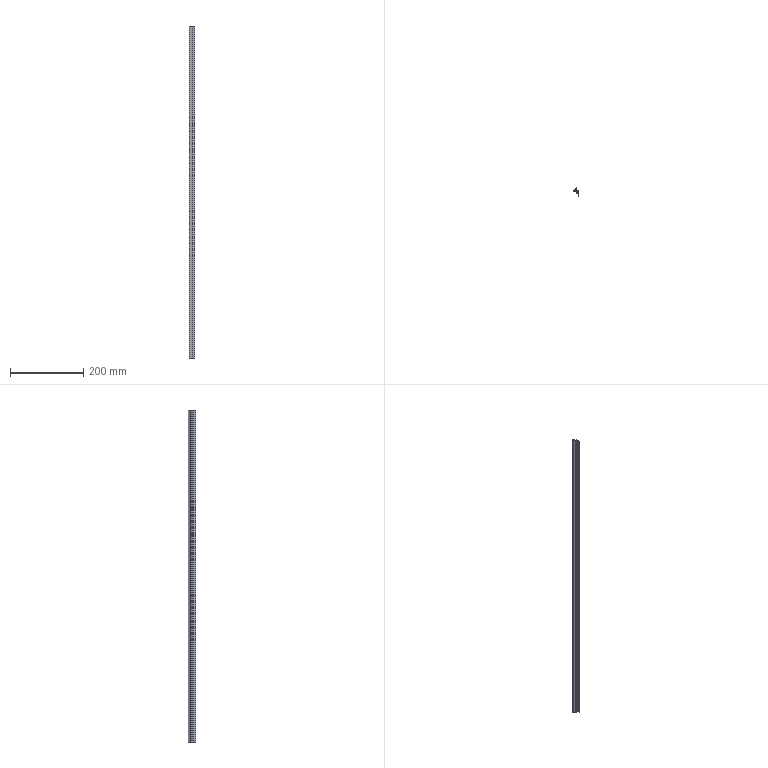Part | SolidWorks | features BaseBody 1, ICE 1, MoveFace 1 | 1 solid | 27 faces | box 14 x 20.3 x 906 mm | volume 46130 mm3 | plane 20 | cylinder 7 | commonest cylinder face diameters 0.387 x2 0.8 x2 0.4 x1 20 x1 22 x1
STEP:
#1=CARTESIAN_POINT('',(-5.304,-0.625,200.));
#2=VERTEX_POINT('',#1);
#3=CARTESIAN_POINT('',(-5.449,-0.8125,200.));
#4=VERTEX_POINT('',#3);
#5=CARTESIAN_POINT('',(-5.255,-0.8125,200.));
#6=DIRECTION('',(0.,0.,1.));
#7=DIRECTION('',(-1.,0.,0.));
#8=AXIS2_PLACEMENT_3D('',#5,#6,#7);
#9=CIRCLE('',#8,0.1937);
#10=EDGE_CURVE('',#2,#4,#9,.T.);
#11=ORIENTED_EDGE('',*,*,#10,.T.);
#12=CARTESIAN_POINT('',(-5.449,-0.8125,-706.));
#13=VERTEX_POINT('',#12);
#14=CARTESIAN_POINT('',(-5.449,-0.8125,230.));
#15=DIRECTION('',(0.,0.,-1.));
#16=VECTOR('',#15,1000.);
#17=LINE('',#14,#16);
#18=EDGE_CURVE('',#4,#13,#17,.T.);
#19=ORIENTED_EDGE('',*,*,#18,.T.);
#20=CARTESIAN_POINT('',(-5.304,-0.625,-706.));
#21=VERTEX_POINT('',#20);
#22=CARTESIAN_POINT('',(-5.255,-0.8125,-706.));
#23=DIRECTION('',(0.,0.,-1.));
#24=DIRECTION('',(1.,0.,0.));
#25=AXIS2_PLACEMENT_3D('',#22,#23,#24);
#26=CIRCLE('',#25,0.1937);
#27=EDGE_CURVE('',#13,#21,#26,.T.);
#28=ORIENTED_EDGE('',*,*,#27,.T.);
#29=CARTESIAN_POINT('',(-5.304,-0.625,230.));
#30=DIRECTION('',(0.,0.,-1.));
#31=VECTOR('',#30,1000.);
#32=LINE('',#29,#31);
#33=EDGE_CURVE('',#2,#21,#32,.T.);
#34=ORIENTED_EDGE('',*,*,#33,.F.);
#35=EDGE_LOOP('',(#11,#19,#28,#34));
#36=FACE_OUTER_BOUND('',#35,.T.);
#37=CARTESIAN_POINT('',(-5.255,-0.8125,230.));
#38=DIRECTION('',(0.,0.,-1.));
#39=DIRECTION('',(-1.,0.,0.));
#40=AXIS2_PLACEMENT_3D('',#37,#38,#39);
#41=CYLINDRICAL_SURFACE('',#40,0.1937);
#42=ADVANCED_FACE('',(#36),#41,.F.);
#43=CARTESIAN_POINT('',(5.,-1.,-706.));
#44=VERTEX_POINT('',#43);
#45=CARTESIAN_POINT('',(5.,-14.3,-706.));
#46=VERTEX_POINT('',#45);
#47=CARTESIAN_POINT('',(5.,29.623,-706.));
#48=DIRECTION('',(0.,-1.,0.));
#49=VECTOR('',#48,1000.);
#50=LINE('',#47,#49);
#51=EDGE_CURVE('',#44,#46,#50,.T.);
#52=ORIENTED_EDGE('',*,*,#51,.F.);
#53=CARTESIAN_POINT('',(5.,-1.,200.));
#54=VERTEX_POINT('',#53);
#55=CARTESIAN_POINT('',(5.,-1.,230.));
#56=DIRECTION('',(0.,0.,-1.));
#57=VECTOR('',#56,1000.);
#58=LINE('',#55,#57);
#59=EDGE_CURVE('',#54,#44,#58,.T.);
#60=ORIENTED_EDGE('',*,*,#59,.F.);
#61=CARTESIAN_POINT('',(5.,-14.3,200.));
#62=VERTEX_POINT('',#61);
#63=CARTESIAN_POINT('',(5.,-14.3,200.));
#64=DIRECTION('',(0.,1.,0.));
#65=VECTOR('',#64,1000.);
#66=LINE('',#63,#65);
#67=EDGE_CURVE('',#62,#54,#66,.T.);
#68=ORIENTED_EDGE('',*,*,#67,.F.);
#69=CARTESIAN_POINT('',(5.,-14.3,230.));
#70=DIRECTION('',(0.,0.,1.));
#71=VECTOR('',#70,1000.);
#72=LINE('',#69,#71);
#73=EDGE_CURVE('',#46,#62,#72,.T.);
#74=ORIENTED_EDGE('',*,*,#73,.F.);
#75=EDGE_LOOP('',(#52,#60,#68,#74));
#76=FACE_OUTER_BOUND('',#75,.T.);
#77=CARTESIAN_POINT('',(5.,-14.3,230.));
#78=DIRECTION('',(-1.,0.,0.));
#79=DIRECTION('',(0.,0.,1.));
#80=AXIS2_PLACEMENT_3D('',#77,#78,#79);
#81=PLANE('',#80);
#82=ADVANCED_FACE('',(#76),#81,.F.);
#83=CARTESIAN_POINT('',(-9.,-2.,-706.));
#84=VERTEX_POINT('',#83);
#85=CARTESIAN_POINT('',(-9.,-2.,200.));
#86=VERTEX_POINT('',#85);
#87=CARTESIAN_POINT('',(-9.,-2.,230.));
#88=DIRECTION('',(0.,0.,1.));
#89=VECTOR('',#88,1000.);
#90=LINE('',#87,#89);
#91=EDGE_CURVE('',#84,#86,#90,.T.);
#92=ORIENTED_EDGE('',*,*,#91,.F.);
#93=CARTESIAN_POINT('',(0.9,-2.,-706.));
#94=VERTEX_POINT('',#93);
#95=CARTESIAN_POINT('',(5.,-2.,-706.));
#96=DIRECTION('',(-1.,0.,0.));
#97=VECTOR('',#96,1000.);
#98=LINE('',#95,#97);
#99=EDGE_CURVE('',#94,#84,#98,.T.);
#100=ORIENTED_EDGE('',*,*,#99,.F.);
#101=CARTESIAN_POINT('',(0.9,-2.,200.));
#102=VERTEX_POINT('',#101);
#103=CARTESIAN_POINT('',(0.9,-2.,230.));
#104=DIRECTION('',(0.,0.,-1.));
#105=VECTOR('',#104,1000.);
#106=LINE('',#103,#105);
#107=EDGE_CURVE('',#102,#94,#106,.T.);
#108=ORIENTED_EDGE('',*,*,#107,.F.);
#109=CARTESIAN_POINT('',(5.,-2.,200.));
#110=DIRECTION('',(1.,0.,0.));
#111=VECTOR('',#110,1000.);
#112=LINE('',#109,#111);
#113=EDGE_CURVE('',#86,#102,#112,.T.);
#114=ORIENTED_EDGE('',*,*,#113,.F.);
#115=EDGE_LOOP('',(#92,#100,#108,#114));
#116=FACE_OUTER_BOUND('',#115,.T.);
#117=CARTESIAN_POINT('',(-9.,-2.,230.));
#118=DIRECTION('',(0.,1.,0.));
#119=DIRECTION('',(0.,0.,1.));
#120=AXIS2_PLACEMENT_3D('',#117,#118,#119);
#121=PLANE('',#120);
#122=ADVANCED_FACE('',(#116),#121,.F.);
#123=CARTESIAN_POINT('',(4.,-6.,200.));
#124=VERTEX_POINT('',#123);
#125=CARTESIAN_POINT('',(4.,-3.,200.));
#126=VERTEX_POINT('',#125);
#127=CARTESIAN_POINT('',(4.,29.623,200.));
#128=DIRECTION('',(0.,1.,0.));
#129=VECTOR('',#128,1000.);
#130=LINE('',#127,#129);
#131=EDGE_CURVE('',#124,#126,#130,.T.);
#132=ORIENTED_EDGE('',*,*,#131,.F.);
#133=CARTESIAN_POINT('',(1.,-6.,200.));
#134=VERTEX_POINT('',#133);
#135=CARTESIAN_POINT('',(5.,-6.,200.));
#136=DIRECTION('',(1.,0.,0.));
#137=VECTOR('',#136,1000.);
#138=LINE('',#135,#137);
#139=EDGE_CURVE('',#134,#124,#138,.T.);
#140=ORIENTED_EDGE('',*,*,#139,.F.);
#141=CARTESIAN_POINT('',(1.,-6.7,200.));
#142=VERTEX_POINT('',#141);
#143=CARTESIAN_POINT('',(1.,-6.,200.));
#144=DIRECTION('',(0.,-1.,0.));
#145=VECTOR('',#144,1000.);
#146=LINE('',#143,#145);
#147=EDGE_CURVE('',#134,#142,#146,.T.);
#148=ORIENTED_EDGE('',*,*,#147,.T.);
#149=CARTESIAN_POINT('',(-1.7,-6.7,200.));
#150=VERTEX_POINT('',#149);
#151=CARTESIAN_POINT('',(5.,-6.7,200.));
#152=DIRECTION('',(1.,0.,0.));
#153=VECTOR('',#152,1000.);
#154=LINE('',#151,#153);
#155=EDGE_CURVE('',#150,#142,#154,.T.);
#156=ORIENTED_EDGE('',*,*,#155,.F.);
#157=CARTESIAN_POINT('',(-1.7,-7.7,200.));
#158=VERTEX_POINT('',#157);
#159=CARTESIAN_POINT('',(-1.7,-6.7,200.));
#160=DIRECTION('',(0.,-1.,0.));
#161=VECTOR('',#160,1000.);
#162=LINE('',#159,#161);
#163=EDGE_CURVE('',#150,#158,#162,.T.);
#164=ORIENTED_EDGE('',*,*,#163,.T.);
#165=CARTESIAN_POINT('',(4.,-7.7,200.));
#166=VERTEX_POINT('',#165);
#167=CARTESIAN_POINT('',(5.,-7.7,200.));
#168=DIRECTION('',(-1.,0.,0.));
#169=VECTOR('',#168,1000.);
#170=LINE('',#167,#169);
#171=EDGE_CURVE('',#166,#158,#170,.T.);
#172=ORIENTED_EDGE('',*,*,#171,.F.);
#173=CARTESIAN_POINT('',(4.,-14.3,200.));
#174=VERTEX_POINT('',#173);
#175=CARTESIAN_POINT('',(4.,29.623,200.));
#176=DIRECTION('',(0.,1.,0.));
#177=VECTOR('',#176,1000.);
#178=LINE('',#175,#177);
#179=EDGE_CURVE('',#174,#166,#178,.T.);
#180=ORIENTED_EDGE('',*,*,#179,.F.);
#181=CARTESIAN_POINT('',(5.,-14.3,200.));
#182=DIRECTION('',(-1.,0.,0.));
#183=VECTOR('',#182,1000.);
#184=LINE('',#181,#183);
#185=EDGE_CURVE('',#62,#174,#184,.T.);
#186=ORIENTED_EDGE('',*,*,#185,.F.);
#187=ORIENTED_EDGE('',*,*,#67,.T.);
#188=CARTESIAN_POINT('',(-5.207,-1.,200.));
#189=VERTEX_POINT('',#188);
#190=CARTESIAN_POINT('',(5.,-1.,200.));
#191=DIRECTION('',(1.,0.,0.));
#192=VECTOR('',#191,1000.);
#193=LINE('',#190,#192);
#194=EDGE_CURVE('',#189,#54,#193,.T.);
#195=ORIENTED_EDGE('',*,*,#194,.F.);
#196=CARTESIAN_POINT('',(-5.255,-0.8125,200.));
#197=DIRECTION('',(0.,0.,1.));
#198=DIRECTION('',(-1.,0.,0.));
#199=AXIS2_PLACEMENT_3D('',#196,#197,#198);
#200=CIRCLE('',#199,0.1937);
#201=EDGE_CURVE('',#4,#189,#200,.T.);
#202=ORIENTED_EDGE('',*,*,#201,.F.);
#203=ORIENTED_EDGE('',*,*,#10,.F.);
#204=CARTESIAN_POINT('',(-1.368,3.063,200.));
#205=VERTEX_POINT('',#204);
#206=CARTESIAN_POINT('',(-10.628,9.,200.));
#207=DIRECTION('',(0.,0.,1.));
#208=DIRECTION('',(-1.,0.,0.));
#209=AXIS2_PLACEMENT_3D('',#206,#207,#208);
#210=CIRCLE('',#209,11.);
#211=EDGE_CURVE('',#2,#205,#210,.T.);
#212=ORIENTED_EDGE('',*,*,#211,.T.);
#213=CARTESIAN_POINT('',(-1.,2.955,200.));
#214=VERTEX_POINT('',#213);
#215=CARTESIAN_POINT('',(-1.2,2.955,200.));
#216=DIRECTION('',(0.,0.,1.));
#217=DIRECTION('',(-1.,0.,0.));
#218=AXIS2_PLACEMENT_3D('',#215,#216,#217);
#219=CIRCLE('',#218,0.2);
#220=EDGE_CURVE('',#214,#205,#219,.T.);
#221=ORIENTED_EDGE('',*,*,#220,.F.);
#222=CARTESIAN_POINT('',(-1.,1.5,200.));
#223=VERTEX_POINT('',#222);
#224=CARTESIAN_POINT('',(-1.,2.955,200.));
#225=DIRECTION('',(0.,1.,0.));
#226=VECTOR('',#225,1000.);
#227=LINE('',#224,#226);
#228=EDGE_CURVE('',#223,#214,#227,.T.);
#229=ORIENTED_EDGE('',*,*,#228,.F.);
#230=CARTESIAN_POINT('',(0.,1.5,200.));
#231=VERTEX_POINT('',#230);
#232=CARTESIAN_POINT('',(-1.,1.5,200.));
#233=DIRECTION('',(-1.,0.,0.));
#234=VECTOR('',#233,1000.);
#235=LINE('',#232,#234);
#236=EDGE_CURVE('',#231,#223,#235,.T.);
#237=ORIENTED_EDGE('',*,*,#236,.F.);
#238=CARTESIAN_POINT('',(0.,6.,200.));
#239=VERTEX_POINT('',#238);
#240=CARTESIAN_POINT('',(0.,1.5,200.));
#241=DIRECTION('',(0.,-1.,0.));
#242=VECTOR('',#241,1000.);
#243=LINE('',#240,#242);
#244=EDGE_CURVE('',#239,#231,#243,.T.);
#245=ORIENTED_EDGE('',*,*,#244,.F.);
#246=CARTESIAN_POINT('',(-0.8,6.,200.));
#247=VERTEX_POINT('',#246);
#248=CARTESIAN_POINT('',(0.,6.,200.));
#249=DIRECTION('',(1.,0.,0.));
#250=VECTOR('',#249,1000.);
#251=LINE('',#248,#250);
#252=EDGE_CURVE('',#247,#239,#251,.T.);
#253=ORIENTED_EDGE('',*,*,#252,.F.);
#254=CARTESIAN_POINT('',(-1.178,5.731,200.));
#255=VERTEX_POINT('',#254);
#256=CARTESIAN_POINT('',(-0.8,5.6,200.));
#257=DIRECTION('',(0.,0.,1.));
#258=DIRECTION('',(-1.,0.,0.));
#259=AXIS2_PLACEMENT_3D('',#256,#257,#258);
#260=CIRCLE('',#259,0.4);
#261=EDGE_CURVE('',#247,#255,#260,.T.);
#262=ORIENTED_EDGE('',*,*,#261,.T.);
#263=CARTESIAN_POINT('',(-8.678,-0.8077,200.));
#264=VERTEX_POINT('',#263);
#265=CARTESIAN_POINT('',(-10.628,9.,200.));
#266=DIRECTION('',(0.,0.,1.));
#267=DIRECTION('',(-1.,0.,0.));
#268=AXIS2_PLACEMENT_3D('',#265,#266,#267);
#269=CIRCLE('',#268,10.);
#270=EDGE_CURVE('',#264,#255,#269,.T.);
#271=ORIENTED_EDGE('',*,*,#270,.F.);
#272=CARTESIAN_POINT('',(-9.,-1.2,200.));
#273=VERTEX_POINT('',#272);
#274=CARTESIAN_POINT('',(-8.6,-1.2,200.));
#275=DIRECTION('',(0.,0.,1.));
#276=DIRECTION('',(-1.,0.,0.));
#277=AXIS2_PLACEMENT_3D('',#274,#275,#276);
#278=CIRCLE('',#277,0.4);
#279=EDGE_CURVE('',#264,#273,#278,.T.);
#280=ORIENTED_EDGE('',*,*,#279,.T.);
#281=CARTESIAN_POINT('',(-9.,8.,200.));
#282=DIRECTION('',(0.,-1.,0.));
#283=VECTOR('',#282,1000.);
#284=LINE('',#281,#283);
#285=EDGE_CURVE('',#273,#86,#284,.T.);
#286=ORIENTED_EDGE('',*,*,#285,.T.);
#287=ORIENTED_EDGE('',*,*,#113,.T.);
#288=CARTESIAN_POINT('',(0.9,-3.,200.));
#289=VERTEX_POINT('',#288);
#290=CARTESIAN_POINT('',(0.9,29.623,200.));
#291=DIRECTION('',(0.,1.,0.));
#292=VECTOR('',#291,1000.);
#293=LINE('',#290,#292);
#294=EDGE_CURVE('',#289,#102,#293,.T.);
#295=ORIENTED_EDGE('',*,*,#294,.F.);
#296=CARTESIAN_POINT('',(5.,-3.,200.));
#297=DIRECTION('',(-1.,0.,0.));
#298=VECTOR('',#297,1000.);
#299=LINE('',#296,#298);
#300=EDGE_CURVE('',#126,#289,#299,.T.);
#301=ORIENTED_EDGE('',*,*,#300,.F.);
#302=EDGE_LOOP('',(#132,#140,#148,#156,#164,#172,#180,#186,#187,#195,#202,#203,#212,#221,#229,#237,#245,#253,#262,#271,#280,#286,#287,#295,#301));
#303=FACE_OUTER_BOUND('',#302,.T.);
#304=CARTESIAN_POINT('',(5.,29.623,200.));
#305=DIRECTION('',(0.,0.,-1.));
#306=DIRECTION('',(-1.,0.,0.));
#307=AXIS2_PLACEMENT_3D('',#304,#305,#306);
#308=PLANE('',#307);
#309=ADVANCED_FACE('',(#303),#308,.F.);
#310=ORIENTED_EDGE('',*,*,#185,.T.);
#311=CARTESIAN_POINT('',(4.,-14.3,-706.));
#312=VERTEX_POINT('',#311);
#313=CARTESIAN_POINT('',(4.,-14.3,230.));
#314=DIRECTION('',(0.,0.,1.));
#315=VECTOR('',#314,1000.);
#316=LINE('',#313,#315);
#317=EDGE_CURVE('',#312,#174,#316,.T.);
#318=ORIENTED_EDGE('',*,*,#317,.F.);
#319=CARTESIAN_POINT('',(5.,-14.3,-706.));
#320=DIRECTION('',(-1.,0.,0.));
#321=VECTOR('',#320,1000.);
#322=LINE('',#319,#321);
#323=EDGE_CURVE('',#46,#312,#322,.T.);
#324=ORIENTED_EDGE('',*,*,#323,.F.);
#325=ORIENTED_EDGE('',*,*,#73,.T.);
#326=EDGE_LOOP('',(#310,#318,#324,#325));
#327=FACE_OUTER_BOUND('',#326,.T.);
#328=CARTESIAN_POINT('',(4.,-14.3,230.));
#329=DIRECTION('',(0.,1.,0.));
#330=DIRECTION('',(0.,0.,1.));
#331=AXIS2_PLACEMENT_3D('',#328,#329,#330);
#332=PLANE('',#331);
#333=ADVANCED_FACE('',(#327),#332,.F.);
#334=ORIENTED_EDGE('',*,*,#51,.T.);
#335=ORIENTED_EDGE('',*,*,#323,.T.);
#336=CARTESIAN_POINT('',(4.,-7.7,-706.));
#337=VERTEX_POINT('',#336);
#338=CARTESIAN_POINT('',(4.,-7.7,-706.));
#339=DIRECTION('',(0.,-1.,0.));
#340=VECTOR('',#339,1000.);
#341=LINE('',#338,#340);
#342=EDGE_CURVE('',#337,#312,#341,.T.);
#343=ORIENTED_EDGE('',*,*,#342,.F.);
#344=CARTESIAN_POINT('',(-1.7,-7.7,-706.));
#345=VERTEX_POINT('',#344);
#346=CARTESIAN_POINT('',(-1.7,-7.7,-706.));
#347=DIRECTION('',(1.,0.,0.));
#348=VECTOR('',#347,1000.);
#349=LINE('',#346,#348);
#350=EDGE_CURVE('',#345,#337,#349,.T.);
#351=ORIENTED_EDGE('',*,*,#350,.F.);
#352=CARTESIAN_POINT('',(-1.7,-6.7,-706.));
#353=VERTEX_POINT('',#352);
#354=CARTESIAN_POINT('',(-1.7,29.623,-706.));
#355=DIRECTION('',(0.,1.,0.));
#356=VECTOR('',#355,1000.);
#357=LINE('',#354,#356);
#358=EDGE_CURVE('',#345,#353,#357,.T.);
#359=ORIENTED_EDGE('',*,*,#358,.T.);
#360=CARTESIAN_POINT('',(1.,-6.7,-706.));
#361=VERTEX_POINT('',#360);
#362=CARTESIAN_POINT('',(1.,-6.7,-706.));
#363=DIRECTION('',(-1.,0.,0.));
#364=VECTOR('',#363,1000.);
#365=LINE('',#362,#364);
#366=EDGE_CURVE('',#361,#353,#365,.T.);
#367=ORIENTED_EDGE('',*,*,#366,.F.);
#368=CARTESIAN_POINT('',(1.,-6.,-706.));
#369=VERTEX_POINT('',#368);
#370=CARTESIAN_POINT('',(1.,29.623,-706.));
#371=DIRECTION('',(0.,1.,0.));
#372=VECTOR('',#371,1000.);
#373=LINE('',#370,#372);
#374=EDGE_CURVE('',#361,#369,#373,.T.);
#375=ORIENTED_EDGE('',*,*,#374,.T.);
#376=CARTESIAN_POINT('',(4.,-6.,-706.));
#377=VERTEX_POINT('',#376);
#378=CARTESIAN_POINT('',(4.,-6.,-706.));
#379=DIRECTION('',(-1.,0.,0.));
#380=VECTOR('',#379,1000.);
#381=LINE('',#378,#380);
#382=EDGE_CURVE('',#377,#369,#381,.T.);
#383=ORIENTED_EDGE('',*,*,#382,.F.);
#384=CARTESIAN_POINT('',(4.,-3.,-706.));
#385=VERTEX_POINT('',#384);
#386=CARTESIAN_POINT('',(4.,-3.,-706.));
#387=DIRECTION('',(0.,-1.,0.));
#388=VECTOR('',#387,1000.);
#389=LINE('',#386,#388);
#390=EDGE_CURVE('',#385,#377,#389,.T.);
#391=ORIENTED_EDGE('',*,*,#390,.F.);
#392=CARTESIAN_POINT('',(0.9,-3.,-706.));
#393=VERTEX_POINT('',#392);
#394=CARTESIAN_POINT('',(0.9,-3.,-706.));
#395=DIRECTION('',(1.,0.,0.));
#396=VECTOR('',#395,1000.);
#397=LINE('',#394,#396);
#398=EDGE_CURVE('',#393,#385,#397,.T.);
#399=ORIENTED_EDGE('',*,*,#398,.F.);
#400=CARTESIAN_POINT('',(0.9,-2.,-706.));
#401=DIRECTION('',(0.,-1.,0.));
#402=VECTOR('',#401,1000.);
#403=LINE('',#400,#402);
#404=EDGE_CURVE('',#94,#393,#403,.T.);
#405=ORIENTED_EDGE('',*,*,#404,.F.);
#406=ORIENTED_EDGE('',*,*,#99,.T.);
#407=CARTESIAN_POINT('',(-9.,-1.2,-706.));
#408=VERTEX_POINT('',#407);
#409=CARTESIAN_POINT('',(-9.,-1.2,-706.));
#410=DIRECTION('',(0.,-1.,0.));
#411=VECTOR('',#410,1000.);
#412=LINE('',#409,#411);
#413=EDGE_CURVE('',#408,#84,#412,.T.);
#414=ORIENTED_EDGE('',*,*,#413,.F.);
#415=CARTESIAN_POINT('',(-8.678,-0.8077,-706.));
#416=VERTEX_POINT('',#415);
#417=CARTESIAN_POINT('',(-8.6,-1.2,-706.));
#418=DIRECTION('',(0.,0.,-1.));
#419=DIRECTION('',(1.,0.,0.));
#420=AXIS2_PLACEMENT_3D('',#417,#418,#419);
#421=CIRCLE('',#420,0.4);
#422=EDGE_CURVE('',#408,#416,#421,.T.);
#423=ORIENTED_EDGE('',*,*,#422,.T.);
#424=CARTESIAN_POINT('',(-1.178,5.731,-706.));
#425=VERTEX_POINT('',#424);
#426=CARTESIAN_POINT('',(-10.628,9.,-706.));
#427=DIRECTION('',(0.,0.,-1.));
#428=DIRECTION('',(1.,0.,0.));
#429=AXIS2_PLACEMENT_3D('',#426,#427,#428);
#430=CIRCLE('',#429,10.);
#431=EDGE_CURVE('',#425,#416,#430,.T.);
#432=ORIENTED_EDGE('',*,*,#431,.F.);
#433=CARTESIAN_POINT('',(-0.8,6.,-706.));
#434=VERTEX_POINT('',#433);
#435=CARTESIAN_POINT('',(-0.8,5.6,-706.));
#436=DIRECTION('',(0.,0.,-1.));
#437=DIRECTION('',(1.,0.,0.));
#438=AXIS2_PLACEMENT_3D('',#435,#436,#437);
#439=CIRCLE('',#438,0.4);
#440=EDGE_CURVE('',#425,#434,#439,.T.);
#441=ORIENTED_EDGE('',*,*,#440,.T.);
#442=CARTESIAN_POINT('',(0.,6.,-706.));
#443=VERTEX_POINT('',#442);
#444=CARTESIAN_POINT('',(0.,6.,-706.));
#445=DIRECTION('',(-1.,0.,0.));
#446=VECTOR('',#445,1000.);
#447=LINE('',#444,#446);
#448=EDGE_CURVE('',#443,#434,#447,.T.);
#449=ORIENTED_EDGE('',*,*,#448,.F.);
#450=CARTESIAN_POINT('',(0.,1.5,-706.));
#451=VERTEX_POINT('',#450);
#452=CARTESIAN_POINT('',(0.,1.5,-706.));
#453=DIRECTION('',(0.,1.,0.));
#454=VECTOR('',#453,1000.);
#455=LINE('',#452,#454);
#456=EDGE_CURVE('',#451,#443,#455,.T.);
#457=ORIENTED_EDGE('',*,*,#456,.F.);
#458=CARTESIAN_POINT('',(-1.,1.5,-706.));
#459=VERTEX_POINT('',#458);
#460=CARTESIAN_POINT('',(-1.,1.5,-706.));
#461=DIRECTION('',(1.,0.,0.));
#462=VECTOR('',#461,1000.);
#463=LINE('',#460,#462);
#464=EDGE_CURVE('',#459,#451,#463,.T.);
#465=ORIENTED_EDGE('',*,*,#464,.F.);
#466=CARTESIAN_POINT('',(-1.,2.955,-706.));
#467=VERTEX_POINT('',#466);
#468=CARTESIAN_POINT('',(-1.,2.955,-706.));
#469=DIRECTION('',(0.,-1.,0.));
#470=VECTOR('',#469,1000.);
#471=LINE('',#468,#470);
#472=EDGE_CURVE('',#467,#459,#471,.T.);
#473=ORIENTED_EDGE('',*,*,#472,.F.);
#474=CARTESIAN_POINT('',(-1.368,3.063,-706.));
#475=VERTEX_POINT('',#474);
#476=CARTESIAN_POINT('',(-1.2,2.955,-706.));
#477=DIRECTION('',(0.,0.,-1.));
#478=DIRECTION('',(1.,0.,0.));
#479=AXIS2_PLACEMENT_3D('',#476,#477,#478);
#480=CIRCLE('',#479,0.2);
#481=EDGE_CURVE('',#475,#467,#480,.T.);
#482=ORIENTED_EDGE('',*,*,#481,.F.);
#483=CARTESIAN_POINT('',(-10.628,9.,-706.));
#484=DIRECTION('',(0.,0.,-1.));
#485=DIRECTION('',(1.,0.,0.));
#486=AXIS2_PLACEMENT_3D('',#483,#484,#485);
#487=CIRCLE('',#486,11.);
#488=EDGE_CURVE('',#475,#21,#487,.T.);
#489=ORIENTED_EDGE('',*,*,#488,.T.);
#490=ORIENTED_EDGE('',*,*,#27,.F.);
#491=CARTESIAN_POINT('',(-5.207,-1.,-706.));
#492=VERTEX_POINT('',#491);
#493=CARTESIAN_POINT('',(-5.255,-0.8125,-706.));
#494=DIRECTION('',(0.,0.,-1.));
#495=DIRECTION('',(1.,0.,0.));
#496=AXIS2_PLACEMENT_3D('',#493,#494,#495);
#497=CIRCLE('',#496,0.1937);
#498=EDGE_CURVE('',#492,#13,#497,.T.);
#499=ORIENTED_EDGE('',*,*,#498,.F.);
#500=CARTESIAN_POINT('',(5.,-1.,-706.));
#501=DIRECTION('',(-1.,0.,0.));
#502=VECTOR('',#501,1000.);
#503=LINE('',#500,#502);
#504=EDGE_CURVE('',#44,#492,#503,.T.);
#505=ORIENTED_EDGE('',*,*,#504,.F.);
#506=EDGE_LOOP('',(#334,#335,#343,#351,#359,#367,#375,#383,#391,#399,#405,#406,#414,#423,#432,#441,#449,#457,#465,#473,#482,#489,#490,#499,#505));
#507=FACE_OUTER_BOUND('',#506,.T.);
#508=CARTESIAN_POINT('',(5.,29.623,-706.));
#509=DIRECTION('',(0.,0.,1.));
#510=DIRECTION('',(1.,0.,0.));
#511=AXIS2_PLACEMENT_3D('',#508,#509,#510);
#512=PLANE('',#511);
#513=ADVANCED_FACE('',(#507),#512,.F.);
#514=ORIENTED_EDGE('',*,*,#59,.T.);
#515=ORIENTED_EDGE('',*,*,#504,.T.);
#516=CARTESIAN_POINT('',(-5.207,-1.,230.));
#517=DIRECTION('',(0.,0.,-1.));
#518=VECTOR('',#517,1000.);
#519=LINE('',#516,#518);
#520=EDGE_CURVE('',#189,#492,#519,.T.);
#521=ORIENTED_EDGE('',*,*,#520,.F.);
#522=ORIENTED_EDGE('',*,*,#194,.T.);
#523=EDGE_LOOP('',(#514,#515,#521,#522));
#524=FACE_OUTER_BOUND('',#523,.T.);
#525=CARTESIAN_POINT('',(5.,-1.,230.));
#526=DIRECTION('',(0.,-1.,0.));
#527=DIRECTION('',(0.,0.,-1.));
#528=AXIS2_PLACEMENT_3D('',#525,#526,#527);
#529=PLANE('',#528);
#530=ADVANCED_FACE('',(#524),#529,.F.);
#531=CARTESIAN_POINT('',(-9.,-1.2,230.));
#532=DIRECTION('',(0.,0.,1.));
#533=VECTOR('',#532,1000.);
#534=LINE('',#531,#533);
#535=EDGE_CURVE('',#408,#273,#534,.T.);
#536=ORIENTED_EDGE('',*,*,#535,.F.);
#537=ORIENTED_EDGE('',*,*,#413,.T.);
#538=ORIENTED_EDGE('',*,*,#91,.T.);
#539=ORIENTED_EDGE('',*,*,#285,.F.);
#540=EDGE_LOOP('',(#536,#537,#538,#539));
#541=FACE_OUTER_BOUND('',#540,.T.);
#542=CARTESIAN_POINT('',(-9.,-1.2,230.));
#543=DIRECTION('',(1.,0.,0.));
#544=DIRECTION('',(0.,0.,-1.));
#545=AXIS2_PLACEMENT_3D('',#542,#543,#544);
#546=PLANE('',#545);
#547=ADVANCED_FACE('',(#541),#546,.F.);
#548=ORIENTED_EDGE('',*,*,#294,.T.);
#549=ORIENTED_EDGE('',*,*,#107,.T.);
#550=ORIENTED_EDGE('',*,*,#404,.T.);
#551=CARTESIAN_POINT('',(0.9,-3.,230.));
#552=DIRECTION('',(0.,0.,-1.));
#553=VECTOR('',#552,1000.);
#554=LINE('',#551,#553);
#555=EDGE_CURVE('',#289,#393,#554,.T.);
#556=ORIENTED_EDGE('',*,*,#555,.F.);
#557=EDGE_LOOP('',(#548,#549,#550,#556));
#558=FACE_OUTER_BOUND('',#557,.T.);
#559=CARTESIAN_POINT('',(0.9,-2.,230.));
#560=DIRECTION('',(1.,0.,0.));
#561=DIRECTION('',(0.,0.,-1.));
#562=AXIS2_PLACEMENT_3D('',#559,#560,#561);
#563=PLANE('',#562);
#564=ADVANCED_FACE('',(#558),#563,.F.);
#565=ORIENTED_EDGE('',*,*,#300,.T.);
#566=ORIENTED_EDGE('',*,*,#555,.T.);
#567=ORIENTED_EDGE('',*,*,#398,.T.);
#568=CARTESIAN_POINT('',(4.,-3.,230.));
#569=DIRECTION('',(0.,0.,-1.));
#570=VECTOR('',#569,1000.);
#571=LINE('',#568,#570);
#572=EDGE_CURVE('',#126,#385,#571,.T.);
#573=ORIENTED_EDGE('',*,*,#572,.F.);
#574=EDGE_LOOP('',(#565,#566,#567,#573));
#575=FACE_OUTER_BOUND('',#574,.T.);
#576=CARTESIAN_POINT('',(0.9,-3.,230.));
#577=DIRECTION('',(0.,1.,0.));
#578=DIRECTION('',(0.,0.,1.));
#579=AXIS2_PLACEMENT_3D('',#576,#577,#578);
#580=PLANE('',#579);
#581=ADVANCED_FACE('',(#575),#580,.F.);
#582=ORIENTED_EDGE('',*,*,#131,.T.);
#583=ORIENTED_EDGE('',*,*,#572,.T.);
#584=ORIENTED_EDGE('',*,*,#390,.T.);
#585=CARTESIAN_POINT('',(4.,-6.,230.));
#586=DIRECTION('',(0.,0.,-1.));
#587=VECTOR('',#586,1000.);
#588=LINE('',#585,#587);
#589=EDGE_CURVE('',#124,#377,#588,.T.);
#590=ORIENTED_EDGE('',*,*,#589,.F.);
#591=EDGE_LOOP('',(#582,#583,#584,#590));
#592=FACE_OUTER_BOUND('',#591,.T.);
#593=CARTESIAN_POINT('',(4.,-3.,230.));
#594=DIRECTION('',(1.,0.,0.));
#595=DIRECTION('',(0.,0.,-1.));
#596=AXIS2_PLACEMENT_3D('',#593,#594,#595);
#597=PLANE('',#596);
#598=ADVANCED_FACE('',(#592),#597,.F.);
#599=ORIENTED_EDGE('',*,*,#139,.T.);
#600=ORIENTED_EDGE('',*,*,#589,.T.);
#601=ORIENTED_EDGE('',*,*,#382,.T.);
#602=CARTESIAN_POINT('',(1.,-6.,230.));
#603=DIRECTION('',(0.,0.,-1.));
#604=VECTOR('',#603,1000.);
#605=LINE('',#602,#604);
#606=EDGE_CURVE('',#134,#369,#605,.T.);
#607=ORIENTED_EDGE('',*,*,#606,.F.);
#608=EDGE_LOOP('',(#599,#600,#601,#607));
#609=FACE_OUTER_BOUND('',#608,.T.);
#610=CARTESIAN_POINT('',(4.,-6.,230.));
#611=DIRECTION('',(0.,-1.,0.));
#612=DIRECTION('',(0.,0.,-1.));
#613=AXIS2_PLACEMENT_3D('',#610,#611,#612);
#614=PLANE('',#613);
#615=ADVANCED_FACE('',(#609),#614,.F.);
#616=ORIENTED_EDGE('',*,*,#155,.T.);
#617=CARTESIAN_POINT('',(1.,-6.7,230.));
#618=DIRECTION('',(0.,0.,1.));
#619=VECTOR('',#618,1000.);
#620=LINE('',#617,#619);
#621=EDGE_CURVE('',#361,#142,#620,.T.);
#622=ORIENTED_EDGE('',*,*,#621,.F.);
#623=ORIENTED_EDGE('',*,*,#366,.T.);
#624=CARTESIAN_POINT('',(-1.7,-6.7,230.));
#625=DIRECTION('',(0.,0.,-1.));
#626=VECTOR('',#625,1000.);
#627=LINE('',#624,#626);
#628=EDGE_CURVE('',#150,#353,#627,.T.);
#629=ORIENTED_EDGE('',*,*,#628,.F.);
#630=EDGE_LOOP('',(#616,#622,#623,#629));
#631=FACE_OUTER_BOUND('',#630,.T.);
#632=CARTESIAN_POINT('',(1.,-6.7,230.));
#633=DIRECTION('',(0.,-1.,0.));
#634=DIRECTION('',(0.,0.,-1.));
#635=AXIS2_PLACEMENT_3D('',#632,#633,#634);
#636=PLANE('',#635);
#637=ADVANCED_FACE('',(#631),#636,.F.);
#638=ORIENTED_EDGE('',*,*,#171,.T.);
#639=CARTESIAN_POINT('',(-1.7,-7.7,230.));
#640=DIRECTION('',(0.,0.,1.));
#641=VECTOR('',#640,1000.);
#642=LINE('',#639,#641);
#643=EDGE_CURVE('',#345,#158,#642,.T.);
#644=ORIENTED_EDGE('',*,*,#643,.F.);
#645=ORIENTED_EDGE('',*,*,#350,.T.);
#646=CARTESIAN_POINT('',(4.,-7.7,230.));
#647=DIRECTION('',(0.,0.,-1.));
#648=VECTOR('',#647,1000.);
#649=LINE('',#646,#648);
#650=EDGE_CURVE('',#166,#337,#649,.T.);
#651=ORIENTED_EDGE('',*,*,#650,.F.);
#652=EDGE_LOOP('',(#638,#644,#645,#651));
#653=FACE_OUTER_BOUND('',#652,.T.);
#654=CARTESIAN_POINT('',(-1.7,-7.7,230.));
#655=DIRECTION('',(0.,1.,0.));
#656=DIRECTION('',(0.,0.,1.));
#657=AXIS2_PLACEMENT_3D('',#654,#655,#656);
#658=PLANE('',#657);
#659=ADVANCED_FACE('',(#653),#658,.F.);
#660=ORIENTED_EDGE('',*,*,#179,.T.);
#661=ORIENTED_EDGE('',*,*,#650,.T.);
#662=ORIENTED_EDGE('',*,*,#342,.T.);
#663=ORIENTED_EDGE('',*,*,#317,.T.);
#664=EDGE_LOOP('',(#660,#661,#662,#663));
#665=FACE_OUTER_BOUND('',#664,.T.);
#666=CARTESIAN_POINT('',(4.,-7.7,230.));
#667=DIRECTION('',(1.,0.,0.));
#668=DIRECTION('',(0.,0.,-1.));
#669=AXIS2_PLACEMENT_3D('',#666,#667,#668);
#670=PLANE('',#669);
#671=ADVANCED_FACE('',(#665),#670,.F.);
#672=ORIENTED_EDGE('',*,*,#18,.F.);
#673=ORIENTED_EDGE('',*,*,#201,.T.);
#674=ORIENTED_EDGE('',*,*,#520,.T.);
#675=ORIENTED_EDGE('',*,*,#498,.T.);
#676=EDGE_LOOP('',(#672,#673,#674,#675));
#677=FACE_OUTER_BOUND('',#676,.T.);
#678=CARTESIAN_POINT('',(-5.255,-0.8125,230.));
#679=DIRECTION('',(0.,0.,-1.));
#680=DIRECTION('',(-1.,0.,0.));
#681=AXIS2_PLACEMENT_3D('',#678,#679,#680);
#682=CYLINDRICAL_SURFACE('',#681,0.1937);
#683=ADVANCED_FACE('',(#677),#682,.F.);
#684=CARTESIAN_POINT('',(-1.,2.955,230.));
#685=DIRECTION('',(0.,0.,1.));
#686=VECTOR('',#685,1000.);
#687=LINE('',#684,#686);
#688=EDGE_CURVE('',#467,#214,#687,.T.);
#689=ORIENTED_EDGE('',*,*,#688,.F.);
#690=ORIENTED_EDGE('',*,*,#472,.T.);
#691=CARTESIAN_POINT('',(-1.,1.5,230.));
#692=DIRECTION('',(0.,0.,-1.));
#693=VECTOR('',#692,1000.);
#694=LINE('',#691,#693);
#695=EDGE_CURVE('',#223,#459,#694,.T.);
#696=ORIENTED_EDGE('',*,*,#695,.F.);
#697=ORIENTED_EDGE('',*,*,#228,.T.);
#698=EDGE_LOOP('',(#689,#690,#696,#697));
#699=FACE_OUTER_BOUND('',#698,.T.);
#700=CARTESIAN_POINT('',(-1.,2.955,230.));
#701=DIRECTION('',(1.,0.,0.));
#702=DIRECTION('',(0.,0.,-1.));
#703=AXIS2_PLACEMENT_3D('',#700,#701,#702);
#704=PLANE('',#703);
#705=ADVANCED_FACE('',(#699),#704,.F.);
#706=ORIENTED_EDGE('',*,*,#488,.F.);
#707=CARTESIAN_POINT('',(-1.368,3.063,230.));
#708=DIRECTION('',(0.,0.,1.));
#709=VECTOR('',#708,1000.);
#710=LINE('',#707,#709);
#711=EDGE_CURVE('',#475,#205,#710,.T.);
#712=ORIENTED_EDGE('',*,*,#711,.T.);
#713=ORIENTED_EDGE('',*,*,#211,.F.);
#714=ORIENTED_EDGE('',*,*,#33,.T.);
#715=EDGE_LOOP('',(#706,#712,#713,#714));
#716=FACE_OUTER_BOUND('',#715,.T.);
#717=CARTESIAN_POINT('',(-10.628,9.,230.));
#718=DIRECTION('',(0.,0.,-1.));
#719=DIRECTION('',(-1.,0.,0.));
#720=AXIS2_PLACEMENT_3D('',#717,#718,#719);
#721=CYLINDRICAL_SURFACE('',#720,11.);
#722=ADVANCED_FACE('',(#716),#721,.T.);
#723=CARTESIAN_POINT('',(-1.178,5.731,230.));
#724=DIRECTION('',(0.,0.,1.));
#725=VECTOR('',#724,1000.);
#726=LINE('',#723,#725);
#727=EDGE_CURVE('',#425,#255,#726,.T.);
#728=ORIENTED_EDGE('',*,*,#727,.F.);
#729=ORIENTED_EDGE('',*,*,#431,.T.);
#730=CARTESIAN_POINT('',(-8.678,-0.8077,230.));
#731=DIRECTION('',(0.,0.,-1.));
#732=VECTOR('',#731,1000.);
#733=LINE('',#730,#732);
#734=EDGE_CURVE('',#264,#416,#733,.T.);
#735=ORIENTED_EDGE('',*,*,#734,.F.);
#736=ORIENTED_EDGE('',*,*,#270,.T.);
#737=EDGE_LOOP('',(#728,#729,#735,#736));
#738=FACE_OUTER_BOUND('',#737,.T.);
#739=CARTESIAN_POINT('',(-10.628,9.,230.));
#740=DIRECTION('',(0.,0.,-1.));
#741=DIRECTION('',(-1.,0.,0.));
#742=AXIS2_PLACEMENT_3D('',#739,#740,#741);
#743=CYLINDRICAL_SURFACE('',#742,10.);
#744=ADVANCED_FACE('',(#738),#743,.F.);
#745=CARTESIAN_POINT('',(0.,1.5,230.));
#746=DIRECTION('',(0.,0.,1.));
#747=VECTOR('',#746,1000.);
#748=LINE('',#745,#747);
#749=EDGE_CURVE('',#451,#231,#748,.T.);
#750=ORIENTED_EDGE('',*,*,#749,.F.);
#751=ORIENTED_EDGE('',*,*,#456,.T.);
#752=CARTESIAN_POINT('',(0.,6.,230.));
#753=DIRECTION('',(0.,0.,-1.));
#754=VECTOR('',#753,1000.);
#755=LINE('',#752,#754);
#756=EDGE_CURVE('',#239,#443,#755,.T.);
#757=ORIENTED_EDGE('',*,*,#756,.F.);
#758=ORIENTED_EDGE('',*,*,#244,.T.);
#759=EDGE_LOOP('',(#750,#751,#757,#758));
#760=FACE_OUTER_BOUND('',#759,.T.);
#761=CARTESIAN_POINT('',(0.,1.5,230.));
#762=DIRECTION('',(-1.,0.,0.));
#763=DIRECTION('',(0.,0.,1.));
#764=AXIS2_PLACEMENT_3D('',#761,#762,#763);
#765=PLANE('',#764);
#766=ADVANCED_FACE('',(#760),#765,.F.);
#767=ORIENTED_EDGE('',*,*,#422,.F.);
#768=ORIENTED_EDGE('',*,*,#535,.T.);
#769=ORIENTED_EDGE('',*,*,#279,.F.);
#770=ORIENTED_EDGE('',*,*,#734,.T.);
#771=EDGE_LOOP('',(#767,#768,#769,#770));
#772=FACE_OUTER_BOUND('',#771,.T.);
#773=CARTESIAN_POINT('',(-8.6,-1.2,230.));
#774=DIRECTION('',(0.,0.,-1.));
#775=DIRECTION('',(-1.,0.,0.));
#776=AXIS2_PLACEMENT_3D('',#773,#774,#775);
#777=CYLINDRICAL_SURFACE('',#776,0.4);
#778=ADVANCED_FACE('',(#772),#777,.T.);
#779=ORIENTED_EDGE('',*,*,#147,.F.);
#780=ORIENTED_EDGE('',*,*,#606,.T.);
#781=ORIENTED_EDGE('',*,*,#374,.F.);
#782=ORIENTED_EDGE('',*,*,#621,.T.);
#783=EDGE_LOOP('',(#779,#780,#781,#782));
#784=FACE_OUTER_BOUND('',#783,.T.);
#785=CARTESIAN_POINT('',(1.,-6.,230.));
#786=DIRECTION('',(1.,0.,0.));
#787=DIRECTION('',(0.,0.,-1.));
#788=AXIS2_PLACEMENT_3D('',#785,#786,#787);
#789=PLANE('',#788);
#790=ADVANCED_FACE('',(#784),#789,.F.);
#791=ORIENTED_EDGE('',*,*,#163,.F.);
#792=ORIENTED_EDGE('',*,*,#628,.T.);
#793=ORIENTED_EDGE('',*,*,#358,.F.);
#794=ORIENTED_EDGE('',*,*,#643,.T.);
#795=EDGE_LOOP('',(#791,#792,#793,#794));
#796=FACE_OUTER_BOUND('',#795,.T.);
#797=CARTESIAN_POINT('',(-1.7,-6.7,230.));
#798=DIRECTION('',(1.,0.,0.));
#799=DIRECTION('',(0.,0.,-1.));
#800=AXIS2_PLACEMENT_3D('',#797,#798,#799);
#801=PLANE('',#800);
#802=ADVANCED_FACE('',(#796),#801,.F.);
#803=ORIENTED_EDGE('',*,*,#711,.F.);
#804=ORIENTED_EDGE('',*,*,#481,.T.);
#805=ORIENTED_EDGE('',*,*,#688,.T.);
#806=ORIENTED_EDGE('',*,*,#220,.T.);
#807=EDGE_LOOP('',(#803,#804,#805,#806));
#808=FACE_OUTER_BOUND('',#807,.T.);
#809=CARTESIAN_POINT('',(-1.2,2.955,230.));
#810=DIRECTION('',(0.,0.,-1.));
#811=DIRECTION('',(-1.,0.,0.));
#812=AXIS2_PLACEMENT_3D('',#809,#810,#811);
#813=CYLINDRICAL_SURFACE('',#812,0.2);
#814=ADVANCED_FACE('',(#808),#813,.F.);
#815=ORIENTED_EDGE('',*,*,#695,.T.);
#816=ORIENTED_EDGE('',*,*,#464,.T.);
#817=ORIENTED_EDGE('',*,*,#749,.T.);
#818=ORIENTED_EDGE('',*,*,#236,.T.);
#819=EDGE_LOOP('',(#815,#816,#817,#818));
#820=FACE_OUTER_BOUND('',#819,.T.);
#821=CARTESIAN_POINT('',(-1.,1.5,230.));
#822=DIRECTION('',(0.,1.,0.));
#823=DIRECTION('',(0.,0.,1.));
#824=AXIS2_PLACEMENT_3D('',#821,#822,#823);
#825=PLANE('',#824);
#826=ADVANCED_FACE('',(#820),#825,.F.);
#827=ORIENTED_EDGE('',*,*,#440,.F.);
#828=ORIENTED_EDGE('',*,*,#727,.T.);
#829=ORIENTED_EDGE('',*,*,#261,.F.);
#830=CARTESIAN_POINT('',(-0.8,6.,230.));
#831=DIRECTION('',(0.,0.,-1.));
#832=VECTOR('',#831,1000.);
#833=LINE('',#830,#832);
#834=EDGE_CURVE('',#247,#434,#833,.T.);
#835=ORIENTED_EDGE('',*,*,#834,.T.);
#836=EDGE_LOOP('',(#827,#828,#829,#835));
#837=FACE_OUTER_BOUND('',#836,.T.);
#838=CARTESIAN_POINT('',(-0.8,5.6,230.));
#839=DIRECTION('',(0.,0.,-1.));
#840=DIRECTION('',(-1.,0.,0.));
#841=AXIS2_PLACEMENT_3D('',#838,#839,#840);
#842=CYLINDRICAL_SURFACE('',#841,0.4);
#843=ADVANCED_FACE('',(#837),#842,.T.);
#844=ORIENTED_EDGE('',*,*,#756,.T.);
#845=ORIENTED_EDGE('',*,*,#448,.T.);
#846=ORIENTED_EDGE('',*,*,#834,.F.);
#847=ORIENTED_EDGE('',*,*,#252,.T.);
#848=EDGE_LOOP('',(#844,#845,#846,#847));
#849=FACE_OUTER_BOUND('',#848,.T.);
#850=CARTESIAN_POINT('',(0.,6.,230.));
#851=DIRECTION('',(0.,-1.,0.));
#852=DIRECTION('',(0.,0.,-1.));
#853=AXIS2_PLACEMENT_3D('',#850,#851,#852);
#854=PLANE('',#853);
#855=ADVANCED_FACE('',(#849),#854,.F.);
#856=CLOSED_SHELL('',(#42,#82,#122,#309,#333,#513,#530,#547,#564,#581,#598,#615,#637,#659,#671,#683,#705,#722,#744,#766,#778,#790,#802,#814,#826,#843,#855));
#857=MANIFOLD_SOLID_BREP('',#856);
#858=CARTESIAN_POINT('',(0.,0.,0.));
#859=DIRECTION('',(0.,0.,1.));
#860=DIRECTION('',(1.,0.,0.));
#861=AXIS2_PLACEMENT_3D('',#858,#859,#860);
#862=(LENGTH_UNIT()NAMED_UNIT(*)SI_UNIT(.MILLI.,.METRE.));
#863=UNCERTAINTY_MEASURE_WITH_UNIT(LENGTH_MEASURE(0.00001),#862,'','');
#864=(NAMED_UNIT(*)PLANE_ANGLE_UNIT()SI_UNIT($,.RADIAN.));
#865=(NAMED_UNIT(*)SI_UNIT($,.STERADIAN.)SOLID_ANGLE_UNIT());
#866=(GEOMETRIC_REPRESENTATION_CONTEXT(3)GLOBAL_UNCERTAINTY_ASSIGNED_CONTEXT((#863))GLOBAL_UNIT_ASSIGNED_CONTEXT((#862,#864,#865))REPRESENTATION_CONTEXT('',''));
#867=ADVANCED_BREP_SHAPE_REPRESENTATION('',(#857,#861),#866);